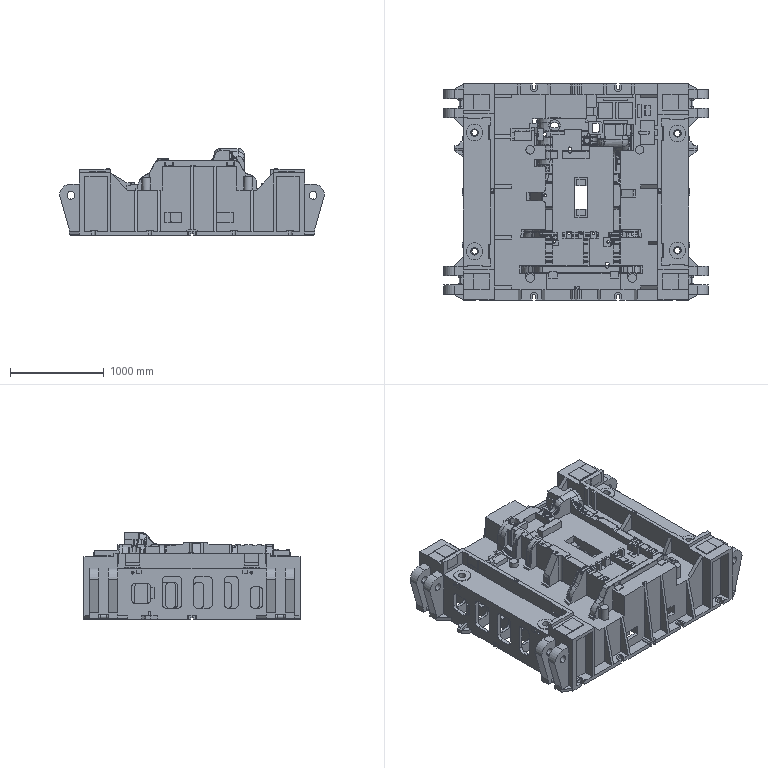Part | NX | features solid 2 | 1 solid | 2916 faces | box 2830 x 2330 x 930.009 mm | volume 1071895023 mm3 | plane 1627 | cylinder 762 | spline 494 | torus 16 | sphere 9 | cone 8 | commonest cylinder face diameters 80 x291 16 x65 20 x61 10 x26 30 x22 32 x20